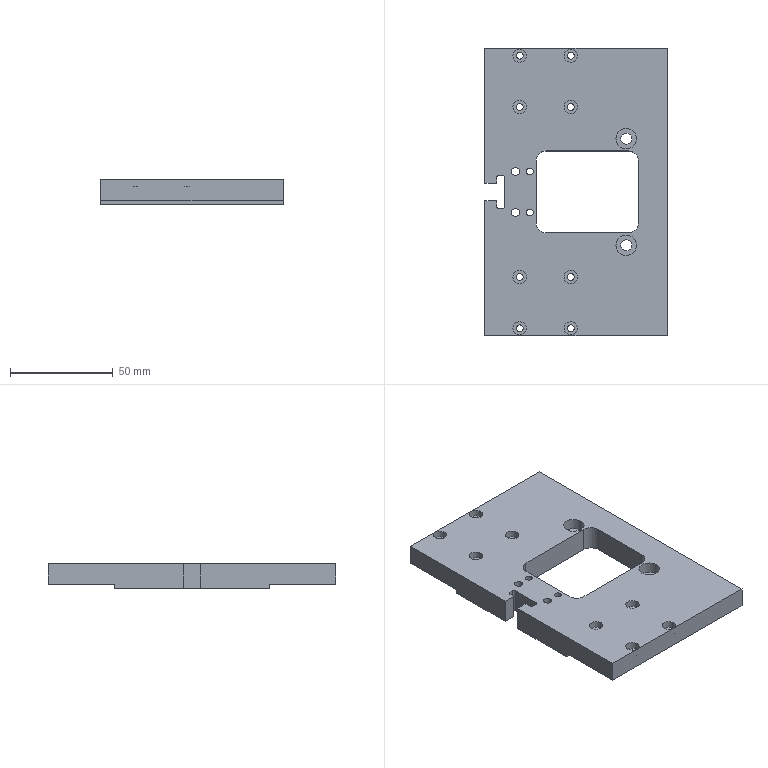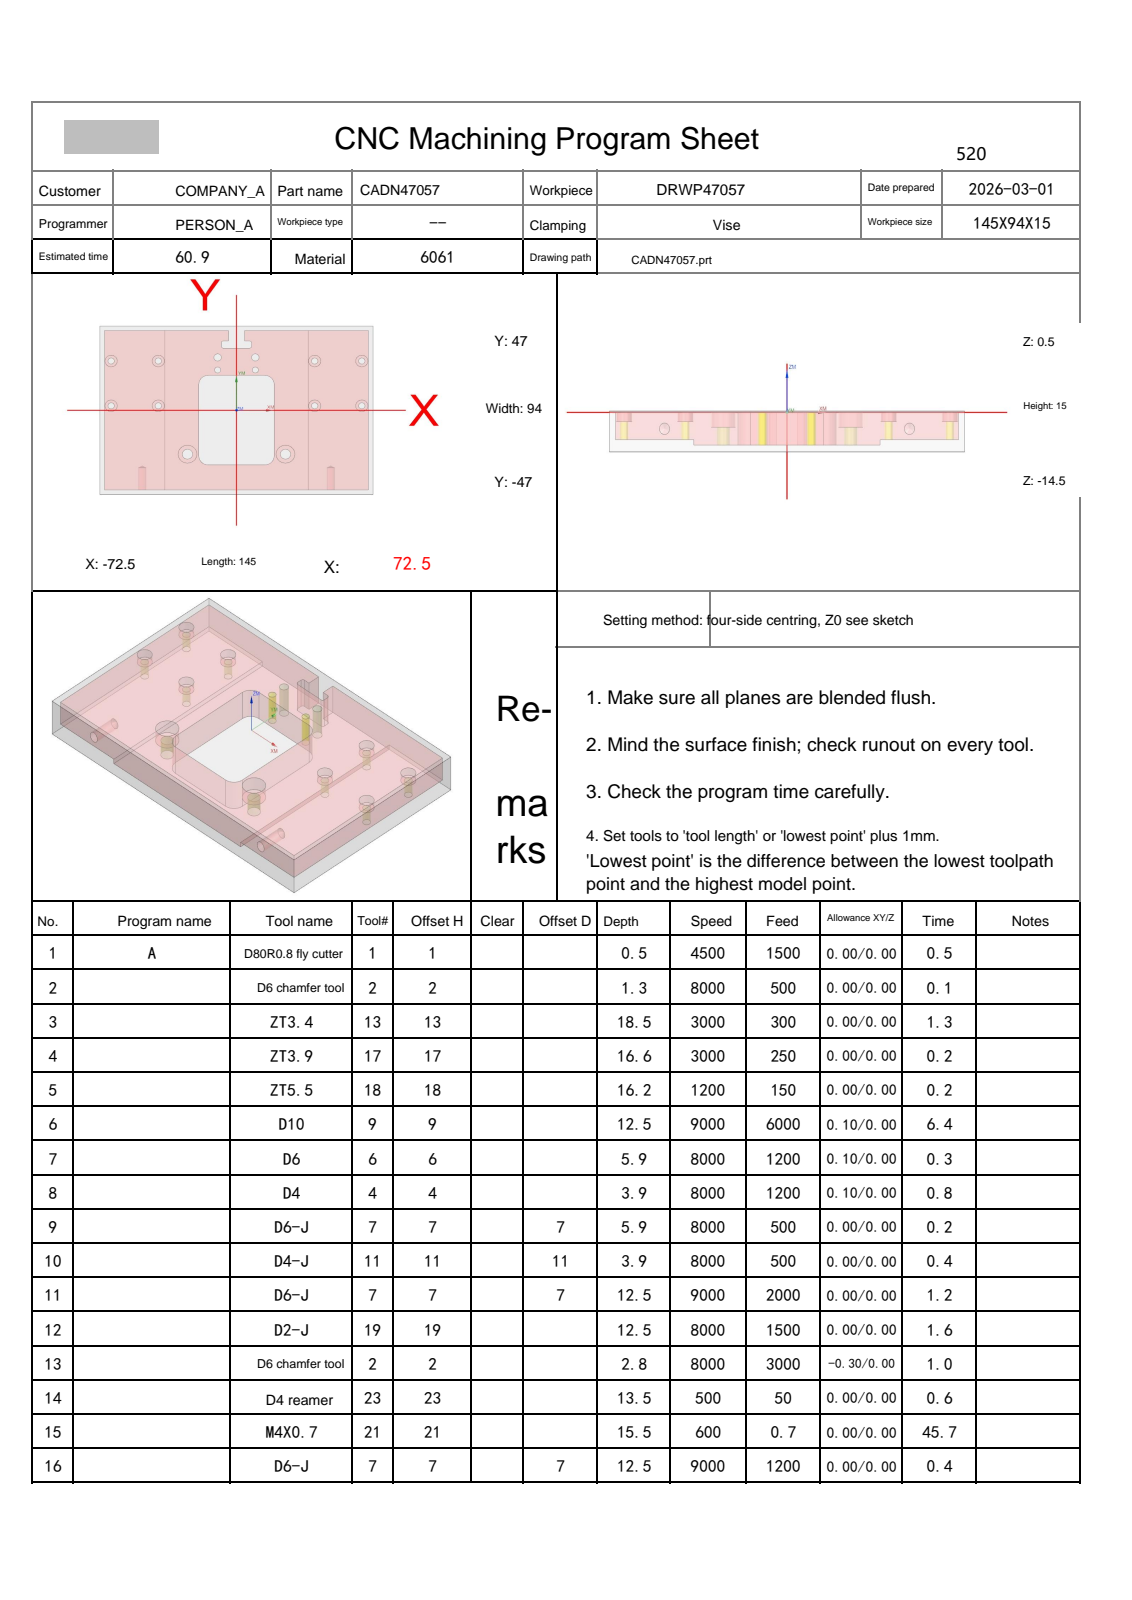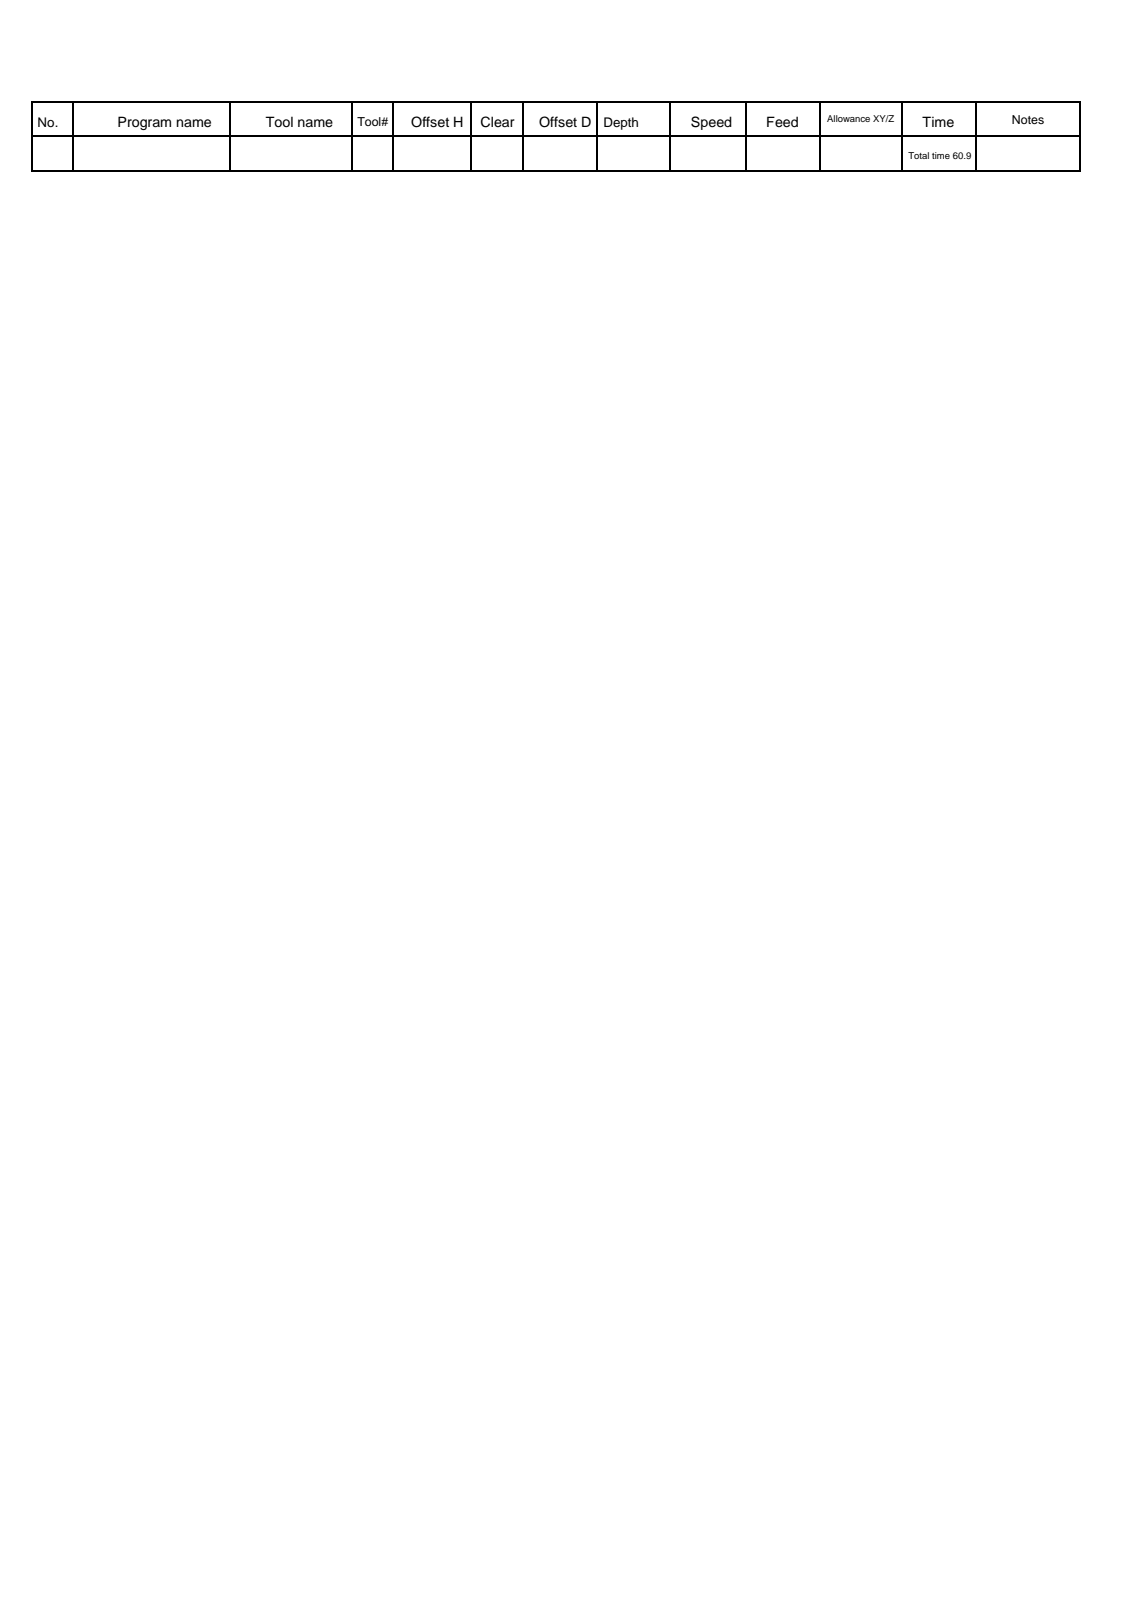NC program | NX | posted by the shop | part box 89 x 140 x 12 mm
Lines 2684 to 3794 of 6684:
N12 T19 M06
(D2-J  D=2. R=0. H=19 ce=0.00 di=0.00)
G00 G90 G54 X-3.031 Y38.716 M03 S8000
G43 H19 Z50.
M08
Z.05
G01 X-3.033 Z.02 F1500.
X-3.041 Y38.715 Z-.008
X-3.052 Y38.714 Z-.032
X-3.067 Y38.711 Z-.054
X-3.085 Y38.708 Z-.073
X-3.105 Y38.703 Z-.09
X-3.126 Y38.696 Z-.104
X-3.148 Y38.687 Z-.116
X-3.17 Y38.676 Z-.126
X-3.191 Y38.662 Z-.134
X-3.211 Y38.646 Z-.14
X-3.228 Y38.627 Z-.145
X-3.243 Y38.604 Z-.148
X-3.254 Y38.578 Z-.149
X-3.262 Y38.549 Z-.15
G02 X-4.25 Y37.7 I-.988 J.151
G01 X-7.
Y35.7
X-1.355
X-1.332 Y35.716 Z-.151
X-1.328 Y35.762 Z-.153
X-1.342 Y35.834 Z-.156
X-1.371 Y35.929 Z-.16
X-1.414 Y36.043 Z-.165
X-1.541 Y36.323 Z-.177
X-1.688 Y36.613 Z-.191
X-1.956 Y37.073 Z-.213
X-2.256 Y37.521 Z-.237
X-2.577 Y37.936 Z-.259
X-2.736 Y38.12 Z-.27
X-2.84 Y38.233 Z-.276
X-2.992 Y38.386 Z-.285
X-3.077 Y38.464 Z-.29
X-3.15 Y38.521 Z-.294
X-3.207 Y38.557 Z-.297
X-3.245 Y38.567 Z-.299
X-3.262 Y38.549 Z-.3
G02 X-4.25 Y37.7 I-.988 J.151
G01 X-7.
Y35.7
X-1.355
X-1.332 Y35.716 Z-.301
X-1.328 Y35.762 Z-.303
X-1.342 Y35.834 Z-.306
X-1.371 Y35.929 Z-.31
X-1.414 Y36.043 Z-.315
X-1.541 Y36.323 Z-.327
X-1.688 Y36.613 Z-.341
X-1.956 Y37.073 Z-.363
X-2.256 Y37.521 Z-.387
X-2.577 Y37.936 Z-.409
X-2.736 Y38.12 Z-.42
X-2.84 Y38.233 Z-.426
X-2.992 Y38.386 Z-.435
X-3.077 Y38.464 Z-.44
X-3.15 Y38.521 Z-.444
X-3.207 Y38.557 Z-.447
X-3.245 Y38.567 Z-.449
X-3.262 Y38.549 Z-.45
G02 X-4.25 Y37.7 I-.988 J.151
G01 X-7.
Y35.7
X-1.355
X-1.332 Y35.716 Z-.451
X-1.328 Y35.762 Z-.453
X-1.342 Y35.834 Z-.456
X-1.371 Y35.929 Z-.46
X-1.414 Y36.043 Z-.465
X-1.541 Y36.323 Z-.477
X-1.688 Y36.613 Z-.491
X-1.956 Y37.073 Z-.513
X-2.256 Y37.521 Z-.537
X-2.577 Y37.936 Z-.559
X-2.736 Y38.12 Z-.57
X-2.84 Y38.233 Z-.576
X-2.992 Y38.386 Z-.585
X-3.077 Y38.464 Z-.59
X-3.15 Y38.521 Z-.594
X-3.207 Y38.557 Z-.597
X-3.245 Y38.567 Z-.599
X-3.262 Y38.549 Z-.6
G02 X-4.25 Y37.7 I-.988 J.151
G01 X-7.
Y35.7
X-1.355
X-1.332 Y35.716 Z-.601
X-1.328 Y35.762 Z-.603
X-1.342 Y35.834 Z-.606
X-1.371 Y35.929 Z-.61
X-1.414 Y36.043 Z-.615
X-1.541 Y36.323 Z-.627
X-1.688 Y36.613 Z-.641
X-1.956 Y37.073 Z-.663
X-2.256 Y37.521 Z-.687
X-2.577 Y37.936 Z-.709
X-2.736 Y38.12 Z-.72
X-2.84 Y38.233 Z-.726
X-2.992 Y38.386 Z-.735
X-3.077 Y38.464 Z-.74
X-3.15 Y38.521 Z-.744
X-3.207 Y38.557 Z-.747
X-3.245 Y38.567 Z-.749
X-3.262 Y38.549 Z-.75
G02 X-4.25 Y37.7 I-.988 J.151
G01 X-7.
Y35.7
X-1.355
X-1.332 Y35.716 Z-.751
X-1.328 Y35.762 Z-.753
X-1.342 Y35.834 Z-.756
X-1.371 Y35.929 Z-.76
X-1.414 Y36.043 Z-.765
X-1.541 Y36.323 Z-.777
X-1.688 Y36.613 Z-.791
X-1.956 Y37.073 Z-.813
X-2.256 Y37.521 Z-.837
X-2.577 Y37.936 Z-.859
X-2.736 Y38.12 Z-.87
X-2.84 Y38.233 Z-.876
X-2.992 Y38.386 Z-.885
X-3.077 Y38.464 Z-.89
X-3.15 Y38.521 Z-.894
X-3.207 Y38.557 Z-.897
X-3.245 Y38.567 Z-.899
X-3.262 Y38.549 Z-.9
G02 X-4.25 Y37.7 I-.988 J.151
G01 X-7.
Y35.7
X-1.355
X-1.332 Y35.716 Z-.901
X-1.328 Y35.762 Z-.903
X-1.342 Y35.834 Z-.906
X-1.371 Y35.929 Z-.91
X-1.414 Y36.043 Z-.915
X-1.541 Y36.323 Z-.927
X-1.688 Y36.613 Z-.941
X-1.956 Y37.073 Z-.963
X-2.256 Y37.521 Z-.987
X-2.577 Y37.936 Z-1.009
X-2.736 Y38.12 Z-1.02
X-2.84 Y38.233 Z-1.026
X-2.992 Y38.386 Z-1.035
X-3.077 Y38.464 Z-1.04
X-3.15 Y38.521 Z-1.044
X-3.207 Y38.557 Z-1.047
X-3.245 Y38.567 Z-1.049
X-3.262 Y38.549 Z-1.05
G02 X-4.25 Y37.7 I-.988 J.151
G01 X-7.
Y35.7
X-1.355
X-1.332 Y35.716 Z-1.051
X-1.328 Y35.762 Z-1.053
X-1.342 Y35.834 Z-1.056
X-1.371 Y35.929 Z-1.06
X-1.414 Y36.043 Z-1.065
X-1.541 Y36.323 Z-1.077
X-1.688 Y36.613 Z-1.091
X-1.956 Y37.073 Z-1.113
X-2.256 Y37.521 Z-1.137
X-2.577 Y37.936 Z-1.159
X-2.736 Y38.12 Z-1.17
X-2.84 Y38.233 Z-1.176
X-2.992 Y38.386 Z-1.185
X-3.077 Y38.464 Z-1.19
X-3.15 Y38.521 Z-1.194
X-3.207 Y38.557 Z-1.197
X-3.245 Y38.567 Z-1.199
X-3.262 Y38.549 Z-1.2
G02 X-4.25 Y37.7 I-.988 J.151
G01 X-7.
Y35.7
X-1.355
X-1.332 Y35.716 Z-1.201
X-1.328 Y35.762 Z-1.203
X-1.342 Y35.834 Z-1.206
X-1.371 Y35.929 Z-1.21
X-1.414 Y36.043 Z-1.215
X-1.541 Y36.323 Z-1.227
X-1.688 Y36.613 Z-1.241
X-1.956 Y37.073 Z-1.263
X-2.256 Y37.521 Z-1.287
X-2.577 Y37.936 Z-1.309
X-2.736 Y38.12 Z-1.32
X-2.84 Y38.233 Z-1.326
X-2.992 Y38.386 Z-1.335
X-3.077 Y38.464 Z-1.34
X-3.15 Y38.521 Z-1.344
X-3.207 Y38.557 Z-1.347
X-3.245 Y38.567 Z-1.349
X-3.262 Y38.549 Z-1.35
G02 X-4.25 Y37.7 I-.988 J.151
G01 X-7.
Y35.7
X-1.355
X-1.332 Y35.716 Z-1.351
X-1.328 Y35.762 Z-1.353
X-1.342 Y35.834 Z-1.356
X-1.371 Y35.929 Z-1.36
X-1.414 Y36.043 Z-1.365
X-1.541 Y36.323 Z-1.377
X-1.688 Y36.613 Z-1.391
X-1.956 Y37.073 Z-1.413
X-2.256 Y37.521 Z-1.437
X-2.577 Y37.936 Z-1.459
X-2.736 Y38.12 Z-1.47
X-2.84 Y38.233 Z-1.476
X-2.992 Y38.386 Z-1.485
X-3.077 Y38.464 Z-1.49
X-3.15 Y38.521 Z-1.494
X-3.207 Y38.557 Z-1.497
X-3.245 Y38.567 Z-1.499
X-3.262 Y38.549 Z-1.5
G02 X-4.25 Y37.7 I-.988 J.151
G01 X-7.
Y35.7
X-1.355
X-1.332 Y35.716 Z-1.501
X-1.328 Y35.762 Z-1.503
X-1.342 Y35.834 Z-1.506
X-1.371 Y35.929 Z-1.51
X-1.414 Y36.043 Z-1.515
X-1.541 Y36.323 Z-1.527
X-1.688 Y36.613 Z-1.541
X-1.956 Y37.073 Z-1.563
X-2.256 Y37.521 Z-1.587
X-2.577 Y37.936 Z-1.609
X-2.736 Y38.12 Z-1.62
X-2.84 Y38.233 Z-1.626
X-2.992 Y38.386 Z-1.635
X-3.077 Y38.464 Z-1.64
X-3.15 Y38.521 Z-1.644
X-3.207 Y38.557 Z-1.647
X-3.245 Y38.567 Z-1.649
X-3.262 Y38.549 Z-1.65
G02 X-4.25 Y37.7 I-.988 J.151
G01 X-7.
Y35.7
X-1.355
X-1.332 Y35.716 Z-1.651
X-1.328 Y35.762 Z-1.653
X-1.342 Y35.834 Z-1.656
X-1.371 Y35.929 Z-1.66
X-1.414 Y36.043 Z-1.665
X-1.541 Y36.323 Z-1.677
X-1.688 Y36.613 Z-1.691
X-1.956 Y37.073 Z-1.713
X-2.256 Y37.521 Z-1.737
X-2.577 Y37.936 Z-1.759
X-2.736 Y38.12 Z-1.77
X-2.84 Y38.233 Z-1.776
X-2.992 Y38.386 Z-1.785
X-3.077 Y38.464 Z-1.79
X-3.15 Y38.521 Z-1.794
X-3.207 Y38.557 Z-1.797
X-3.245 Y38.567 Z-1.799
X-3.262 Y38.549 Z-1.8
G02 X-4.25 Y37.7 I-.988 J.151
G01 X-7.
Y35.7
X-1.355
X-1.332 Y35.716 Z-1.801
X-1.328 Y35.762 Z-1.803
X-1.342 Y35.834 Z-1.806
X-1.371 Y35.929 Z-1.81
X-1.414 Y36.043 Z-1.815
X-1.541 Y36.323 Z-1.827
X-1.688 Y36.613 Z-1.841
X-1.956 Y37.073 Z-1.863
X-2.256 Y37.521 Z-1.887
X-2.577 Y37.936 Z-1.909
X-2.736 Y38.12 Z-1.92
X-2.84 Y38.233 Z-1.926
X-2.992 Y38.386 Z-1.935
X-3.077 Y38.464 Z-1.94
X-3.15 Y38.521 Z-1.944
X-3.207 Y38.557 Z-1.947
X-3.245 Y38.567 Z-1.949
X-3.262 Y38.549 Z-1.95
G02 X-4.25 Y37.7 I-.988 J.151
G01 X-7.
Y35.7
X-1.355
X-1.332 Y35.716 Z-1.951
X-1.328 Y35.762 Z-1.953
X-1.342 Y35.834 Z-1.956
X-1.371 Y35.929 Z-1.96
X-1.414 Y36.043 Z-1.965
X-1.541 Y36.323 Z-1.977
X-1.688 Y36.613 Z-1.991
X-1.956 Y37.073 Z-2.013
X-2.256 Y37.521 Z-2.037
X-2.577 Y37.936 Z-2.059
X-2.736 Y38.12 Z-2.07
X-2.84 Y38.233 Z-2.076
X-2.992 Y38.386 Z-2.085
X-3.077 Y38.464 Z-2.09
X-3.15 Y38.521 Z-2.094
X-3.207 Y38.557 Z-2.097
X-3.245 Y38.567 Z-2.099
X-3.262 Y38.549 Z-2.1
G02 X-4.25 Y37.7 I-.988 J.151
G01 X-7.
Y35.7
X-1.355
X-1.332 Y35.716 Z-2.101
X-1.328 Y35.762 Z-2.103
X-1.342 Y35.834 Z-2.106
X-1.371 Y35.929 Z-2.11
X-1.414 Y36.043 Z-2.115
X-1.541 Y36.323 Z-2.127
X-1.688 Y36.613 Z-2.141
X-1.956 Y37.073 Z-2.163
X-2.256 Y37.521 Z-2.187
X-2.577 Y37.936 Z-2.209
X-2.736 Y38.12 Z-2.22
X-2.84 Y38.233 Z-2.226
X-2.992 Y38.386 Z-2.235
X-3.077 Y38.464 Z-2.24
X-3.15 Y38.521 Z-2.244
X-3.207 Y38.557 Z-2.247
X-3.245 Y38.567 Z-2.249
X-3.262 Y38.549 Z-2.25
G02 X-4.25 Y37.7 I-.988 J.151
G01 X-7.
Y35.7
X-1.355
X-1.332 Y35.716 Z-2.251
X-1.328 Y35.762 Z-2.253
X-1.342 Y35.834 Z-2.256
X-1.371 Y35.929 Z-2.26
X-1.414 Y36.043 Z-2.265
X-1.541 Y36.323 Z-2.277
X-1.688 Y36.613 Z-2.291
X-1.956 Y37.073 Z-2.313
X-2.256 Y37.521 Z-2.337
X-2.577 Y37.936 Z-2.359
X-2.736 Y38.12 Z-2.37
X-2.84 Y38.233 Z-2.376
X-2.992 Y38.386 Z-2.385
X-3.077 Y38.464 Z-2.39
X-3.15 Y38.521 Z-2.394
X-3.207 Y38.557 Z-2.397
X-3.245 Y38.567 Z-2.399
X-3.262 Y38.549 Z-2.4
G02 X-4.25 Y37.7 I-.988 J.151
G01 X-7.
Y35.7
X-1.355
X-1.332 Y35.716 Z-2.401
X-1.328 Y35.762 Z-2.403
X-1.342 Y35.834 Z-2.406
X-1.371 Y35.929 Z-2.41
X-1.414 Y36.043 Z-2.415
X-1.541 Y36.323 Z-2.427
X-1.688 Y36.613 Z-2.441
X-1.956 Y37.073 Z-2.463
X-2.256 Y37.521 Z-2.487
X-2.577 Y37.936 Z-2.509
X-2.736 Y38.12 Z-2.52
X-2.84 Y38.233 Z-2.526
X-2.992 Y38.386 Z-2.535
X-3.077 Y38.464 Z-2.54
X-3.15 Y38.521 Z-2.544
X-3.207 Y38.557 Z-2.547
X-3.245 Y38.567 Z-2.549
X-3.262 Y38.549 Z-2.55
G02 X-4.25 Y37.7 I-.988 J.151
G01 X-7.
Y35.7
X-1.355
X-1.332 Y35.716 Z-2.551
X-1.328 Y35.762 Z-2.553
X-1.342 Y35.834 Z-2.556
X-1.371 Y35.929 Z-2.56
X-1.414 Y36.043 Z-2.565
X-1.541 Y36.323 Z-2.577
X-1.688 Y36.613 Z-2.591
X-1.956 Y37.073 Z-2.613
X-2.256 Y37.521 Z-2.637
X-2.577 Y37.936 Z-2.659
X-2.736 Y38.12 Z-2.67
X-2.84 Y38.233 Z-2.676
X-2.992 Y38.386 Z-2.685
X-3.077 Y38.464 Z-2.69
X-3.15 Y38.521 Z-2.694
X-3.207 Y38.557 Z-2.697
X-3.245 Y38.567 Z-2.699
X-3.262 Y38.549 Z-2.7
G02 X-4.25 Y37.7 I-.988 J.151
G01 X-7.
Y35.7
X-1.355
X-1.332 Y35.716 Z-2.701
X-1.328 Y35.762 Z-2.703
X-1.342 Y35.834 Z-2.706
X-1.371 Y35.929 Z-2.71
X-1.414 Y36.043 Z-2.715
X-1.541 Y36.323 Z-2.727
X-1.688 Y36.613 Z-2.741
X-1.956 Y37.073 Z-2.763
X-2.256 Y37.521 Z-2.787
X-2.577 Y37.936 Z-2.809
X-2.736 Y38.12 Z-2.82
X-2.84 Y38.233 Z-2.826
X-2.992 Y38.386 Z-2.835
X-3.077 Y38.464 Z-2.84
X-3.15 Y38.521 Z-2.844
X-3.207 Y38.557 Z-2.847
X-3.245 Y38.567 Z-2.849
X-3.262 Y38.549 Z-2.85
G02 X-4.25 Y37.7 I-.988 J.151
G01 X-7.
Y35.7
X-1.355
X-1.332 Y35.716 Z-2.851
X-1.328 Y35.762 Z-2.853
X-1.342 Y35.834 Z-2.856
X-1.371 Y35.929 Z-2.86
X-1.414 Y36.043 Z-2.865
X-1.541 Y36.323 Z-2.877
X-1.688 Y36.613 Z-2.891
X-1.956 Y37.073 Z-2.913
X-2.256 Y37.521 Z-2.937
X-2.577 Y37.936 Z-2.959
X-2.736 Y38.12 Z-2.97
X-2.84 Y38.233 Z-2.976
X-2.992 Y38.386 Z-2.985
X-3.077 Y38.464 Z-2.99
X-3.15 Y38.521 Z-2.994
X-3.207 Y38.557 Z-2.997
X-3.245 Y38.567 Z-2.999
X-3.262 Y38.549 Z-3.
G02 X-4.25 Y37.7 I-.988 J.151
G01 X-7.
Y35.7
X-1.355
X-1.332 Y35.716 Z-3.001
X-1.328 Y35.762 Z-3.003
X-1.342 Y35.834 Z-3.006
X-1.371 Y35.929 Z-3.01
X-1.414 Y36.043 Z-3.015
X-1.541 Y36.323 Z-3.027
X-1.688 Y36.613 Z-3.041
X-1.956 Y37.073 Z-3.063
X-2.256 Y37.521 Z-3.087
X-2.577 Y37.936 Z-3.109
X-2.736 Y38.12 Z-3.12
X-2.84 Y38.233 Z-3.126
X-2.992 Y38.386 Z-3.135
X-3.077 Y38.464 Z-3.14
X-3.15 Y38.521 Z-3.144
X-3.207 Y38.557 Z-3.147
X-3.245 Y38.567 Z-3.149
X-3.262 Y38.549 Z-3.15
G02 X-4.25 Y37.7 I-.988 J.151
G01 X-7.
Y35.7
X-1.355
X-1.332 Y35.716 Z-3.151
X-1.328 Y35.762 Z-3.153
X-1.342 Y35.834 Z-3.156
X-1.371 Y35.929 Z-3.16
X-1.414 Y36.043 Z-3.165
X-1.541 Y36.323 Z-3.177
X-1.688 Y36.613 Z-3.191
X-1.956 Y37.073 Z-3.213
X-2.256 Y37.521 Z-3.237
X-2.577 Y37.936 Z-3.259
X-2.736 Y38.12 Z-3.27
X-2.84 Y38.233 Z-3.276
X-2.992 Y38.386 Z-3.285
X-3.077 Y38.464 Z-3.29
X-3.15 Y38.521 Z-3.294
X-3.207 Y38.557 Z-3.297
X-3.245 Y38.567 Z-3.299
X-3.262 Y38.549 Z-3.3
G02 X-4.25 Y37.7 I-.988 J.151
G01 X-7.
Y35.7
X-1.355
X-1.332 Y35.716 Z-3.301
X-1.328 Y35.762 Z-3.303
X-1.342 Y35.834 Z-3.306
X-1.371 Y35.929 Z-3.31
X-1.414 Y36.043 Z-3.315
X-1.541 Y36.323 Z-3.327
X-1.688 Y36.613 Z-3.341
X-1.956 Y37.073 Z-3.363
X-2.256 Y37.521 Z-3.387
X-2.577 Y37.936 Z-3.409
X-2.736 Y38.12 Z-3.42
X-2.84 Y38.233 Z-3.426
X-2.992 Y38.386 Z-3.435
X-3.077 Y38.464 Z-3.44
X-3.15 Y38.521 Z-3.444
X-3.207 Y38.557 Z-3.447
X-3.245 Y38.567 Z-3.449
X-3.262 Y38.549 Z-3.45
G02 X-4.25 Y37.7 I-.988 J.151
G01 X-7.
Y35.7
X-1.355
X-1.332 Y35.716 Z-3.451
X-1.328 Y35.762 Z-3.453
X-1.342 Y35.834 Z-3.456
X-1.371 Y35.929 Z-3.46
X-1.414 Y36.043 Z-3.465
X-1.541 Y36.323 Z-3.477
X-1.688 Y36.613 Z-3.491
X-1.956 Y37.073 Z-3.513
X-2.256 Y37.521 Z-3.537
X-2.577 Y37.936 Z-3.559
X-2.736 Y38.12 Z-3.57
X-2.84 Y38.233 Z-3.576
X-2.992 Y38.386 Z-3.585
X-3.077 Y38.464 Z-3.59
X-3.15 Y38.521 Z-3.594
X-3.207 Y38.557 Z-3.597
X-3.245 Y38.567 Z-3.599
X-3.262 Y38.549 Z-3.6
G02 X-4.25 Y37.7 I-.988 J.151
G01 X-7.
Y35.7
X-1.355
X-1.332 Y35.716 Z-3.601
X-1.328 Y35.762 Z-3.603
X-1.342 Y35.834 Z-3.606
X-1.371 Y35.929 Z-3.61
X-1.414 Y36.043 Z-3.615
X-1.541 Y36.323 Z-3.627
X-1.688 Y36.613 Z-3.641
X-1.956 Y37.073 Z-3.663
X-2.256 Y37.521 Z-3.687
X-2.577 Y37.936 Z-3.709
X-2.736 Y38.12 Z-3.72
X-2.84 Y38.233 Z-3.726
X-2.992 Y38.386 Z-3.735
X-3.077 Y38.464 Z-3.74
X-3.15 Y38.521 Z-3.744
X-3.207 Y38.557 Z-3.747
X-3.245 Y38.567 Z-3.749
X-3.262 Y38.549 Z-3.75
G02 X-4.25 Y37.7 I-.988 J.151
G01 X-7.
Y35.7
X-1.355
X-1.332 Y35.716 Z-3.751
X-1.328 Y35.762 Z-3.753
X-1.342 Y35.834 Z-3.756
X-1.371 Y35.929 Z-3.76
X-1.414 Y36.043 Z-3.765
X-1.541 Y36.323 Z-3.777
X-1.688 Y36.613 Z-3.791
X-1.956 Y37.073 Z-3.813
X-2.256 Y37.521 Z-3.837
X-2.577 Y37.936 Z-3.859
X-2.736 Y38.12 Z-3.87
X-2.84 Y38.233 Z-3.876
X-2.992 Y38.386 Z-3.885
X-3.077 Y38.464 Z-3.89
X-3.15 Y38.521 Z-3.894
X-3.207 Y38.557 Z-3.897
X-3.245 Y38.567 Z-3.899
X-3.262 Y38.549 Z-3.9
G02 X-4.25 Y37.7 I-.988 J.151
G01 X-7.
Y35.7
X-1.355
X-1.332 Y35.716 Z-3.901
X-1.328 Y35.762 Z-3.903
X-1.342 Y35.834 Z-3.906
X-1.371 Y35.929 Z-3.91
X-1.414 Y36.043 Z-3.915
X-1.541 Y36.323 Z-3.927
X-1.688 Y36.613 Z-3.941
X-1.956 Y37.073 Z-3.963
X-2.256 Y37.521 Z-3.987
X-2.577 Y37.936 Z-4.009
X-2.736 Y38.12 Z-4.02
X-2.84 Y38.233 Z-4.026
X-2.992 Y38.386 Z-4.035
X-3.077 Y38.464 Z-4.04
X-3.15 Y38.521 Z-4.044
X-3.207 Y38.557 Z-4.047
X-3.245 Y38.567 Z-4.049
X-3.262 Y38.549 Z-4.05
G02 X-4.25 Y37.7 I-.988 J.151
G01 X-7.
Y35.7
X-1.355
X-1.332 Y35.716 Z-4.051
X-1.328 Y35.762 Z-4.053
X-1.342 Y35.834 Z-4.056
X-1.371 Y35.929 Z-4.06
X-1.414 Y36.043 Z-4.065
X-1.541 Y36.323 Z-4.077
X-1.688 Y36.613 Z-4.091
X-1.956 Y37.073 Z-4.113
X-2.256 Y37.521 Z-4.137
X-2.577 Y37.936 Z-4.159
X-2.736 Y38.12 Z-4.17
X-2.84 Y38.233 Z-4.176
X-2.992 Y38.386 Z-4.185
X-3.077 Y38.464 Z-4.19
X-3.15 Y38.521 Z-4.194
X-3.207 Y38.557 Z-4.197
X-3.245 Y38.567 Z-4.199
X-3.262 Y38.549 Z-4.2
G02 X-4.25 Y37.7 I-.988 J.151
G01 X-7.
Y35.7
X-1.355
X-1.332 Y35.716 Z-4.201
X-1.328 Y35.762 Z-4.203
X-1.342 Y35.834 Z-4.206
X-1.371 Y35.929 Z-4.21
X-1.414 Y36.043 Z-4.215
X-1.541 Y36.323 Z-4.227
X-1.688 Y36.613 Z-4.241
X-1.956 Y37.073 Z-4.263
X-2.256 Y37.521 Z-4.287
X-2.577 Y37.936 Z-4.309
X-2.736 Y38.12 Z-4.32
X-2.84 Y38.233 Z-4.326
X-2.992 Y38.386 Z-4.335
X-3.077 Y38.464 Z-4.34
X-3.15 Y38.521 Z-4.344
X-3.207 Y38.557 Z-4.347
X-3.245 Y38.567 Z-4.349
X-3.262 Y38.549 Z-4.35
G02 X-4.25 Y37.7 I-.988 J.151
G01 X-7.
Y35.7
X-1.355
X-1.332 Y35.716 Z-4.351
X-1.328 Y35.762 Z-4.353
X-1.342 Y35.834 Z-4.356
X-1.371 Y35.929 Z-4.36
X-1.414 Y36.043 Z-4.365
X-1.541 Y36.323 Z-4.377
X-1.688 Y36.613 Z-4.391
X-1.956 Y37.073 Z-4.413
X-2.256 Y37.521 Z-4.437
X-2.577 Y37.936 Z-4.459
X-2.736 Y38.12 Z-4.47
X-2.84 Y38.233 Z-4.476
X-2.992 Y38.386 Z-4.485
X-3.077 Y38.464 Z-4.49
X-3.15 Y38.521 Z-4.494
X-3.207 Y38.557 Z-4.497
X-3.245 Y38.567 Z-4.499
X-3.262 Y38.549 Z-4.5
G02 X-4.25 Y37.7 I-.988 J.151
G01 X-7.
Y35.7
X-1.355
X-1.332 Y35.716 Z-4.501
X-1.328 Y35.762 Z-4.503
X-1.342 Y35.834 Z-4.506
X-1.371 Y35.929 Z-4.51
X-1.414 Y36.043 Z-4.515
X-1.541 Y36.323 Z-4.527
X-1.688 Y36.613 Z-4.541
X-1.956 Y37.073 Z-4.563
X-2.256 Y37.521 Z-4.587
X-2.577 Y37.936 Z-4.609
X-2.736 Y38.12 Z-4.62
X-2.84 Y38.233 Z-4.626
X-2.992 Y38.386 Z-4.635
X-3.077 Y38.464 Z-4.64
X-3.15 Y38.521 Z-4.644
X-3.207 Y38.557 Z-4.647
X-3.245 Y38.567 Z-4.649
X-3.262 Y38.549 Z-4.65
G02 X-4.25 Y37.7 I-.988 J.151
G01 X-7.
Y35.7
X-1.355
X-1.332 Y35.716 Z-4.651
X-1.328 Y35.762 Z-4.653
X-1.342 Y35.834 Z-4.656
X-1.371 Y35.929 Z-4.66
X-1.414 Y36.043 Z-4.665
X-1.541 Y36.323 Z-4.677
X-1.688 Y36.613 Z-4.691
X-1.956 Y37.073 Z-4.713
X-2.256 Y37.521 Z-4.737
X-2.577 Y37.936 Z-4.759
X-2.736 Y38.12 Z-4.77
X-2.84 Y38.233 Z-4.776
X-2.992 Y38.386 Z-4.785
X-3.077 Y38.464 Z-4.79
X-3.15 Y38.521 Z-4.794
X-3.207 Y38.557 Z-4.797
X-3.245 Y38.567 Z-4.799
X-3.262 Y38.549 Z-4.8
G02 X-4.25 Y37.7 I-.988 J.151
G01 X-7.
Y35.7
X-1.355
X-1.332 Y35.716 Z-4.801
X-1.328 Y35.762 Z-4.803
X-1.342 Y35.834 Z-4.806
X-1.371 Y35.929 Z-4.81
X-1.414 Y36.043 Z-4.815
X-1.541 Y36.323 Z-4.827
X-1.688 Y36.613 Z-4.841
X-1.956 Y37.073 Z-4.863
X-2.256 Y37.521 Z-4.887
X-2.577 Y37.936 Z-4.909
X-2.736 Y38.12 Z-4.92
X-2.84 Y38.233 Z-4.926
X-2.992 Y38.386 Z-4.935
X-3.077 Y38.464 Z-4.94
X-3.15 Y38.521 Z-4.944
X-3.207 Y38.557 Z-4.947
X-3.245 Y38.567 Z-4.949
X-3.262 Y38.549 Z-4.95
G02 X-4.25 Y37.7 I-.988 J.151
G01 X-7.
Y35.7
X-1.355
X-1.332 Y35.716 Z-4.951
X-1.328 Y35.762 Z-4.953
X-1.342 Y35.834 Z-4.956
X-1.371 Y35.929 Z-4.96
X-1.414 Y36.043 Z-4.965
X-1.541 Y36.323 Z-4.977
X-1.688 Y36.613 Z-4.991
X-1.956 Y37.073 Z-5.013
X-2.256 Y37.521 Z-5.037
X-2.577 Y37.936 Z-5.059
X-2.736 Y38.12 Z-5.07
X-2.84 Y38.233 Z-5.076
X-2.992 Y38.386 Z-5.085
X-3.077 Y38.464 Z-5.09
X-3.15 Y38.521 Z-5.094
X-3.207 Y38.557 Z-5.097
X-3.245 Y38.567 Z-5.099
X-3.262 Y38.549 Z-5.1
G02 X-4.25 Y37.7 I-.988 J.151
G01 X-7.
Y35.7
X-1.355
X-1.332 Y35.716 Z-5.101
X-1.328 Y35.762 Z-5.103
X-1.342 Y35.834 Z-5.106
X-1.371 Y35.929 Z-5.11
X-1.414 Y36.043 Z-5.115
X-1.541 Y36.323 Z-5.127
X-1.688 Y36.613 Z-5.141
X-1.956 Y37.073 Z-5.163
X-2.256 Y37.521 Z-5.187
X-2.577 Y37.936 Z-5.209
X-2.736 Y38.12 Z-5.22
X-2.84 Y38.233 Z-5.226
X-2.992 Y38.386 Z-5.235
X-3.077 Y38.464 Z-5.24
X-3.15 Y38.521 Z-5.244
X-3.207 Y38.557 Z-5.247
X-3.245 Y38.567 Z-5.249
X-3.262 Y38.549 Z-5.25
G02 X-4.25 Y37.7 I-.988 J.151
G01 X-7.
Y35.7
X-1.355
X-1.332 Y35.716 Z-5.251
X-1.328 Y35.762 Z-5.253
X-1.342 Y35.834 Z-5.256
X-1.371 Y35.929 Z-5.26
X-1.414 Y36.043 Z-5.265
X-1.541 Y36.323 Z-5.277
X-1.688 Y36.613 Z-5.291
X-1.956 Y37.073 Z-5.313
X-2.256 Y37.521 Z-5.337
X-2.577 Y37.936 Z-5.359
X-2.736 Y38.12 Z-5.37
X-2.84 Y38.233 Z-5.376
X-2.992 Y38.386 Z-5.385
X-3.077 Y38.464 Z-5.39
X-3.15 Y38.521 Z-5.394
X-3.207 Y38.557 Z-5.397
X-3.245 Y38.567 Z-5.399
X-3.262 Y38.549 Z-5.4
G02 X-4.25 Y37.7 I-.988 J.151
G01 X-7.
Y35.7
X-1.355
X-1.332 Y35.716 Z-5.401
X-1.328 Y35.762 Z-5.403
X-1.342 Y35.834 Z-5.406
X-1.371 Y35.929 Z-5.41
X-1.414 Y36.043 Z-5.415
X-1.541 Y36.323 Z-5.427
X-1.688 Y36.613 Z-5.441
X-1.956 Y37.073 Z-5.463
X-2.256 Y37.521 Z-5.487
X-2.577 Y37.936 Z-5.509
X-2.736 Y38.12 Z-5.52
X-2.84 Y38.233 Z-5.526
X-2.992 Y38.386 Z-5.535
X-3.077 Y38.464 Z-5.54
X-3.15 Y38.521 Z-5.544
X-3.207 Y38.557 Z-5.547
X-3.245 Y38.567 Z-5.549
X-3.262 Y38.549 Z-5.55
G02 X-4.25 Y37.7 I-.988 J.151
G01 X-7.
Y35.7
X-1.355
X-1.332 Y35.716 Z-5.551
X-1.328 Y35.762 Z-5.553
X-1.342 Y35.834 Z-5.556
X-1.371 Y35.929 Z-5.56
X-1.414 Y36.043 Z-5.565
X-1.541 Y36.323 Z-5.577
X-1.688 Y36.613 Z-5.591
X-1.956 Y37.073 Z-5.613
X-2.256 Y37.521 Z-5.637
X-2.577 Y37.936 Z-5.659
X-2.736 Y38.12 Z-5.67
X-2.84 Y38.233 Z-5.676
X-2.992 Y38.386 Z-5.685
X-3.077 Y38.464 Z-5.69
X-3.15 Y38.521 Z-5.694
X-3.207 Y38.557 Z-5.697
X-3.245 Y38.567 Z-5.699
X-3.262 Y38.549 Z-5.7
G02 X-4.25 Y37.7 I-.988 J.151
G01 X-7.
Y35.7
X-1.355
X-1.332 Y35.716 Z-5.701
X-1.328 Y35.762 Z-5.703
X-1.342 Y35.834 Z-5.706
X-1.371 Y35.929 Z-5.71
X-1.414 Y36.043 Z-5.715
X-1.541 Y36.323 Z-5.727
X-1.688 Y36.613 Z-5.741
X-1.956 Y37.073 Z-5.763
X-2.256 Y37.521 Z-5.787
X-2.577 Y37.936 Z-5.809
X-2.736 Y38.12 Z-5.82
X-2.84 Y38.233 Z-5.826
X-2.992 Y38.386 Z-5.835
X-3.077 Y38.464 Z-5.84
X-3.15 Y38.521 Z-5.844
X-3.207 Y38.557 Z-5.847
X-3.245 Y38.567 Z-5.849
X-3.262 Y38.549 Z-5.85
G02 X-4.25 Y37.7 I-.988 J.151
G01 X-7.
Y35.7
X-1.355
X-1.332 Y35.716 Z-5.851
X-1.328 Y35.762 Z-5.853
X-1.342 Y35.834 Z-5.856
X-1.371 Y35.929 Z-5.86
X-1.414 Y36.043 Z-5.865
X-1.541 Y36.323 Z-5.877
X-1.688 Y36.613 Z-5.891
X-1.956 Y37.073 Z-5.913
X-2.256 Y37.521 Z-5.937
X-2.577 Y37.936 Z-5.959
X-2.736 Y38.12 Z-5.97
X-2.84 Y38.233 Z-5.976
X-2.992 Y38.386 Z-5.985
X-3.077 Y38.464 Z-5.99
X-3.15 Y38.521 Z-5.994
X-3.207 Y38.557 Z-5.997
X-3.245 Y38.567 Z-5.999
X-3.262 Y38.549 Z-6.
G02 X-4.25 Y37.7 I-.988 J.151
G01 X-7.
Y35.7
X-1.355
X-1.332 Y35.716 Z-6.001
X-1.328 Y35.762 Z-6.003
X-1.342 Y35.834 Z-6.006
X-1.371 Y35.929 Z-6.01
X-1.414 Y36.043 Z-6.015
X-1.541 Y36.323 Z-6.027
X-1.688 Y36.613 Z-6.041
X-1.956 Y37.073 Z-6.063
X-2.256 Y37.521 Z-6.087
X-2.577 Y37.936 Z-6.109
X-2.736 Y38.12 Z-6.12
X-2.84 Y38.233 Z-6.126
X-2.992 Y38.386 Z-6.135
X-3.077 Y38.464 Z-6.14
X-3.15 Y38.521 Z-6.144
X-3.207 Y38.557 Z-6.147
X-3.245 Y38.567 Z-6.149
X-3.262 Y38.549 Z-6.15
G02 X-4.25 Y37.7 I-.988 J.151
G01 X-7.
Y35.7
X-1.355
X-1.332 Y35.716 Z-6.151
X-1.328 Y35.762 Z-6.153
X-1.342 Y35.834 Z-6.156
X-1.371 Y35.929 Z-6.16
X-1.414 Y36.043 Z-6.165
X-1.541 Y36.323 Z-6.177
X-1.688 Y36.613 Z-6.191
X-1.956 Y37.073 Z-6.213
X-2.256 Y37.521 Z-6.237
X-2.577 Y37.936 Z-6.259
X-2.736 Y38.12 Z-6.27
X-2.84 Y38.233 Z-6.276
X-2.992 Y38.386 Z-6.285
X-3.077 Y38.464 Z-6.29
X-3.15 Y38.521 Z-6.294
X-3.207 Y38.557 Z-6.297
X-3.245 Y38.567 Z-6.299
X-3.262 Y38.549 Z-6.3
G02 X-4.25 Y37.7 I-.988 J.151
G01 X-7.
Y35.7
X-1.355
X-1.332 Y35.716 Z-6.301
X-1.328 Y35.762 Z-6.303
X-1.342 Y35.834 Z-6.306
X-1.371 Y35.929 Z-6.31
X-1.414 Y36.043 Z-6.315
X-1.541 Y36.323 Z-6.327
X-1.688 Y36.613 Z-6.341
X-1.956 Y37.073 Z-6.363
X-2.256 Y37.521 Z-6.387
X-2.577 Y37.936 Z-6.409
X-2.736 Y38.12 Z-6.42
X-2.84 Y38.233 Z-6.426
X-2.992 Y38.386 Z-6.435
X-3.077 Y38.464 Z-6.44
X-3.15 Y38.521 Z-6.444
X-3.207 Y38.557 Z-6.447
X-3.245 Y38.567 Z-6.449
X-3.262 Y38.549 Z-6.45
G02 X-4.25 Y37.7 I-.988 J.151
G01 X-7.
Y35.7
X-1.355
X-1.332 Y35.716 Z-6.451
X-1.328 Y35.762 Z-6.453
X-1.342 Y35.834 Z-6.456
X-1.371 Y35.929 Z-6.46
X-1.414 Y36.043 Z-6.465
X-1.541 Y36.323 Z-6.477
X-1.688 Y36.613 Z-6.491
X-1.956 Y37.073 Z-6.513
X-2.256 Y37.521 Z-6.537
X-2.577 Y37.936 Z-6.559
X-2.736 Y38.12 Z-6.57
X-2.84 Y38.233 Z-6.576
X-2.992 Y38.386 Z-6.585
X-3.077 Y38.464 Z-6.59
X-3.15 Y38.521 Z-6.594
X-3.207 Y38.557 Z-6.597
X-3.245 Y38.567 Z-6.599
X-3.262 Y38.549 Z-6.6
G02 X-4.25 Y37.7 I-.988 J.151
G01 X-7.
Y35.7
X-1.355
X-1.332 Y35.716 Z-6.601
X-1.328 Y35.762 Z-6.603
X-1.342 Y35.834 Z-6.606
X-1.371 Y35.929 Z-6.61
X-1.414 Y36.043 Z-6.615
X-1.541 Y36.323 Z-6.627
X-1.688 Y36.613 Z-6.641
X-1.956 Y37.073 Z-6.663
X-2.256 Y37.521 Z-6.687
X-2.577 Y37.936 Z-6.709
X-2.736 Y38.12 Z-6.72
X-2.84 Y38.233 Z-6.726
X-2.992 Y38.386 Z-6.735
X-3.077 Y38.464 Z-6.74
X-3.15 Y38.521 Z-6.744
X-3.207 Y38.557 Z-6.747
X-3.245 Y38.567 Z-6.749
X-3.262 Y38.549 Z-6.75
G02 X-4.25 Y37.7 I-.988 J.151
G01 X-7.
Y35.7
X-1.355
X-1.332 Y35.716 Z-6.751
X-1.328 Y35.762 Z-6.753
X-1.342 Y35.834 Z-6.756
X-1.371 Y35.929 Z-6.76
X-1.414 Y36.043 Z-6.765
X-1.541 Y36.323 Z-6.777
X-1.688 Y36.613 Z-6.791
X-1.956 Y37.073 Z-6.813
X-2.256 Y37.521 Z-6.837
X-2.577 Y37.936 Z-6.859
X-2.736 Y38.12 Z-6.87
X-2.84 Y38.233 Z-6.876
X-2.992 Y38.386 Z-6.885
X-3.077 Y38.464 Z-6.89
X-3.15 Y38.521 Z-6.894
X-3.207 Y38.557 Z-6.897
X-3.245 Y38.567 Z-6.899
X-3.262 Y38.549 Z-6.9
G02 X-4.25 Y37.7 I-.988 J.151
G01 X-7.
Y35.7
X-1.355
X-1.332 Y35.716 Z-6.901
X-1.328 Y35.762 Z-6.903
X-1.342 Y35.834 Z-6.906
X-1.371 Y35.929 Z-6.91
X-1.414 Y36.043 Z-6.915
X-1.541 Y36.323 Z-6.927
X-1.688 Y36.613 Z-6.941
X-1.956 Y37.073 Z-6.963
X-2.256 Y37.521 Z-6.987
X-2.577 Y37.936 Z-7.009
X-2.736 Y38.12 Z-7.02
X-2.84 Y38.233 Z-7.026
X-2.992 Y38.386 Z-7.035
X-3.077 Y38.464 Z-7.04
X-3.15 Y38.521 Z-7.044
X-3.207 Y38.557 Z-7.047
X-3.245 Y38.567 Z-7.049
X-3.262 Y38.549 Z-7.05
G02 X-4.25 Y37.7 I-.988 J.151
G01 X-7.
Y35.7
X-1.355
X-1.332 Y35.716 Z-7.051
X-1.328 Y35.762 Z-7.053
X-1.342 Y35.834 Z-7.056
X-1.371 Y35.929 Z-7.06
X-1.414 Y36.043 Z-7.065
X-1.541 Y36.323 Z-7.077
X-1.688 Y36.613 Z-7.091
X-1.956 Y37.073 Z-7.113
X-2.256 Y37.521 Z-7.137
X-2.577 Y37.936 Z-7.159
X-2.736 Y38.12 Z-7.17
X-2.84 Y38.233 Z-7.176
X-2.992 Y38.386 Z-7.185
X-3.077 Y38.464 Z-7.19
X-3.15 Y38.521 Z-7.194
X-3.207 Y38.557 Z-7.197
X-3.245 Y38.567 Z-7.199
X-3.262 Y38.549 Z-7.2
G02 X-4.25 Y37.7 I-.988 J.151
G01 X-7.
Y35.7
X-1.355
X-1.332 Y35.716 Z-7.201
X-1.328 Y35.762 Z-7.203
X-1.342 Y35.834 Z-7.206
X-1.371 Y35.929 Z-7.21
X-1.414 Y36.043 Z-7.215
X-1.541 Y36.323 Z-7.227
X-1.688 Y36.613 Z-7.241
X-1.956 Y37.073 Z-7.263
X-2.256 Y37.521 Z-7.287
X-2.577 Y37.936 Z-7.309
X-2.736 Y38.12 Z-7.32
X-2.84 Y38.233 Z-7.326
X-2.992 Y38.386 Z-7.335
X-3.077 Y38.464 Z-7.34
X-3.15 Y38.521 Z-7.344
X-3.207 Y38.557 Z-7.347
X-3.245 Y38.567 Z-7.349
X-3.262 Y38.549 Z-7.35
G02 X-4.25 Y37.7 I-.988 J.151
G01 X-7.
Y35.7
X-1.355
X-1.332 Y35.716 Z-7.351
X-1.328 Y35.762 Z-7.353
X-1.342 Y35.834 Z-7.356
X-1.371 Y35.929 Z-7.36
X-1.414 Y36.043 Z-7.365
X-1.541 Y36.323 Z-7.377
X-1.688 Y36.613 Z-7.391
X-1.956 Y37.073 Z-7.413
X-2.256 Y37.521 Z-7.437
X-2.577 Y37.936 Z-7.459
X-2.736 Y38.12 Z-7.47
X-2.84 Y38.233 Z-7.476
X-2.992 Y38.386 Z-7.485
X-3.077 Y38.464 Z-7.49
X-3.15 Y38.521 Z-7.494
X-3.207 Y38.557 Z-7.497
X-3.245 Y38.567 Z-7.499
X-3.262 Y38.549 Z-7.5
G02 X-4.25 Y37.7 I-.988 J.151
G01 X-7.
Y35.7
X-1.355
X-1.332 Y35.716 Z-7.501
X-1.328 Y35.762 Z-7.503
X-1.342 Y35.834 Z-7.506
X-1.371 Y35.929 Z-7.51
X-1.414 Y36.043 Z-7.515
X-1.541 Y36.323 Z-7.527
X-1.688 Y36.613 Z-7.541
X-1.956 Y37.073 Z-7.563